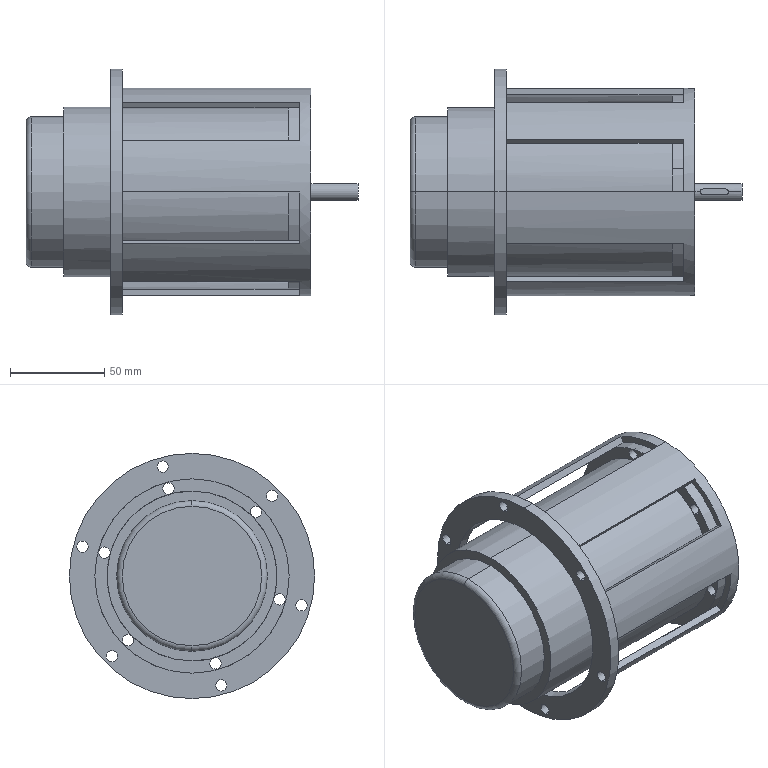Part | NX | features BREP 1 | 1 solid | 75 faces | box 176 x 130 x 130 mm | volume 1047266 mm3 | cylinder 45 | plane 28 | torus 2 | commonest cylinder face diameters 6 x12 6.009 x12 103 x8 3 x3 9 x2 80 x2